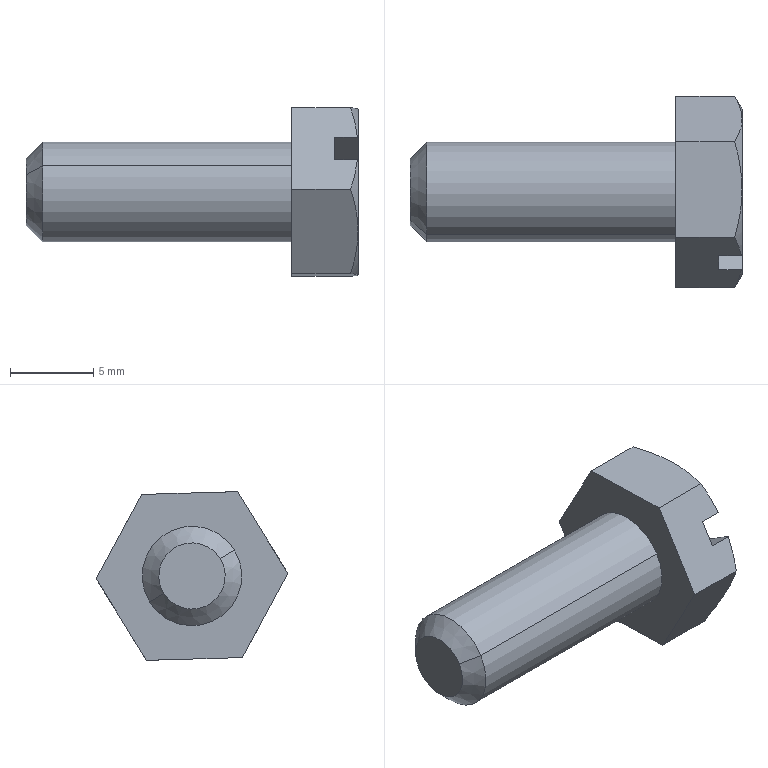Part | SolidWorks | features BaseBody 1 | 1 solid | 23 faces | box 20 x 11.542 x 10.162 mm | volume 766.933 mm3 | plane 13 | cone 8 | cylinder 2 | commonest cylinder face diameters 6 x2
STEP:
#1=CARTESIAN_POINT('',(431.2,61.298,25.05));
#2=VERTEX_POINT('',#1);
#3=CARTESIAN_POINT('',(431.2,64.702,22.95));
#4=VERTEX_POINT('',#3);
#5=CARTESIAN_POINT('',(431.2,63.,24.));
#6=DIRECTION('',(-1.,0.,0.));
#7=DIRECTION('',(0.,-0.8512,0.5248));
#8=AXIS2_PLACEMENT_3D('',#5,#6,#7);
#9=CIRCLE('',#8,2.);
#10=EDGE_CURVE('',#2,#4,#9,.T.);
#11=ORIENTED_EDGE('',*,*,#10,.F.);
#12=CARTESIAN_POINT('',(432.2,60.446,25.574));
#13=VERTEX_POINT('',#12);
#14=CARTESIAN_POINT('',(431.2,61.298,25.05));
#15=DIRECTION('',(0.7071,-0.6019,0.3711));
#16=VECTOR('',#15,1000.);
#17=LINE('',#14,#16);
#18=EDGE_CURVE('',#2,#13,#17,.T.);
#19=ORIENTED_EDGE('',*,*,#18,.T.);
#20=CARTESIAN_POINT('',(432.2,65.554,22.426));
#21=VERTEX_POINT('',#20);
#22=CARTESIAN_POINT('',(432.2,63.,24.));
#23=DIRECTION('',(1.,0.,0.));
#24=DIRECTION('',(0.,-0.8512,0.5248));
#25=AXIS2_PLACEMENT_3D('',#22,#23,#24);
#26=CIRCLE('',#25,3.);
#27=EDGE_CURVE('',#21,#13,#26,.T.);
#28=ORIENTED_EDGE('',*,*,#27,.F.);
#29=CARTESIAN_POINT('',(431.2,64.702,22.95));
#30=DIRECTION('',(0.7071,0.6019,-0.3711));
#31=VECTOR('',#30,1000.);
#32=LINE('',#29,#31);
#33=EDGE_CURVE('',#4,#21,#32,.T.);
#34=ORIENTED_EDGE('',*,*,#33,.F.);
#35=EDGE_LOOP('',(#11,#19,#28,#34));
#36=FACE_OUTER_BOUND('',#35,.T.);
#37=CARTESIAN_POINT('',(431.2,63.,24.));
#38=DIRECTION('',(1.,0.,0.));
#39=DIRECTION('',(0.,0.8512,-0.5248));
#40=AXIS2_PLACEMENT_3D('',#37,#38,#39);
#41=CONICAL_SURFACE('',#40,2.,0.7854);
#42=ADVANCED_FACE('',(#36),#41,.T.);
#43=ORIENTED_EDGE('',*,*,#27,.T.);
#44=CARTESIAN_POINT('',(447.2,60.446,25.574));
#45=VERTEX_POINT('',#44);
#46=CARTESIAN_POINT('',(431.2,60.446,25.574));
#47=DIRECTION('',(1.,0.,0.));
#48=VECTOR('',#47,1000.);
#49=LINE('',#46,#48);
#50=EDGE_CURVE('',#13,#45,#49,.T.);
#51=ORIENTED_EDGE('',*,*,#50,.T.);
#52=CARTESIAN_POINT('',(447.2,65.554,22.426));
#53=VERTEX_POINT('',#52);
#54=CARTESIAN_POINT('',(447.2,63.,24.));
#55=DIRECTION('',(-1.,0.,0.));
#56=DIRECTION('',(0.,-0.8512,0.5248));
#57=AXIS2_PLACEMENT_3D('',#54,#55,#56);
#58=CIRCLE('',#57,3.);
#59=EDGE_CURVE('',#45,#53,#58,.T.);
#60=ORIENTED_EDGE('',*,*,#59,.T.);
#61=CARTESIAN_POINT('',(431.2,65.554,22.426));
#62=DIRECTION('',(1.,0.,0.));
#63=VECTOR('',#62,1000.);
#64=LINE('',#61,#63);
#65=EDGE_CURVE('',#21,#53,#64,.T.);
#66=ORIENTED_EDGE('',*,*,#65,.F.);
#67=EDGE_LOOP('',(#43,#51,#60,#66));
#68=FACE_OUTER_BOUND('',#67,.T.);
#69=CARTESIAN_POINT('',(431.2,63.,24.));
#70=DIRECTION('',(1.,0.,0.));
#71=DIRECTION('',(0.,0.8512,-0.5248));
#72=AXIS2_PLACEMENT_3D('',#69,#70,#71);
#73=CYLINDRICAL_SURFACE('',#72,3.);
#74=ADVANCED_FACE('',(#68),#73,.T.);
#75=CARTESIAN_POINT('',(447.2,66.03,28.915));
#76=VERTEX_POINT('',#75);
#77=CARTESIAN_POINT('',(447.2,68.771,23.833));
#78=VERTEX_POINT('',#77);
#79=CARTESIAN_POINT('',(447.2,68.771,23.833));
#80=DIRECTION('',(0.,0.4748,-0.8801));
#81=VECTOR('',#80,1000.);
#82=LINE('',#79,#81);
#83=EDGE_CURVE('',#76,#78,#82,.T.);
#84=ORIENTED_EDGE('',*,*,#83,.T.);
#85=CARTESIAN_POINT('',(447.2,65.741,18.919));
#86=VERTEX_POINT('',#85);
#87=CARTESIAN_POINT('',(447.2,65.741,18.919));
#88=DIRECTION('',(0.,-0.5248,-0.8512));
#89=VECTOR('',#88,1000.);
#90=LINE('',#87,#89);
#91=EDGE_CURVE('',#78,#86,#90,.T.);
#92=ORIENTED_EDGE('',*,*,#91,.T.);
#93=CARTESIAN_POINT('',(447.2,59.97,19.085));
#94=VERTEX_POINT('',#93);
#95=CARTESIAN_POINT('',(447.2,65.741,18.919));
#96=DIRECTION('',(0.,-0.9996,0.02887));
#97=VECTOR('',#96,1000.);
#98=LINE('',#95,#97);
#99=EDGE_CURVE('',#86,#94,#98,.T.);
#100=ORIENTED_EDGE('',*,*,#99,.T.);
#101=CARTESIAN_POINT('',(447.2,57.229,24.167));
#102=VERTEX_POINT('',#101);
#103=CARTESIAN_POINT('',(447.2,57.229,24.167));
#104=DIRECTION('',(0.,-0.4748,0.8801));
#105=VECTOR('',#104,1000.);
#106=LINE('',#103,#105);
#107=EDGE_CURVE('',#94,#102,#106,.T.);
#108=ORIENTED_EDGE('',*,*,#107,.T.);
#109=CARTESIAN_POINT('',(447.2,60.259,29.081));
#110=VERTEX_POINT('',#109);
#111=CARTESIAN_POINT('',(447.2,57.229,24.167));
#112=DIRECTION('',(0.,0.5248,0.8512));
#113=VECTOR('',#112,1000.);
#114=LINE('',#111,#113);
#115=EDGE_CURVE('',#102,#110,#114,.T.);
#116=ORIENTED_EDGE('',*,*,#115,.T.);
#117=CARTESIAN_POINT('',(447.2,60.259,29.081));
#118=DIRECTION('',(0.,0.9996,-0.02887));
#119=VECTOR('',#118,1000.);
#120=LINE('',#117,#119);
#121=EDGE_CURVE('',#110,#76,#120,.T.);
#122=ORIENTED_EDGE('',*,*,#121,.T.);
#123=EDGE_LOOP('',(#84,#92,#100,#108,#116,#122));
#124=FACE_OUTER_BOUND('',#123,.T.);
#125=CARTESIAN_POINT('',(447.2,63.,24.));
#126=DIRECTION('',(-1.,0.,0.));
#127=DIRECTION('',(0.,-0.8512,0.5248));
#128=AXIS2_PLACEMENT_3D('',#125,#126,#127);
#129=CIRCLE('',#128,3.);
#130=EDGE_CURVE('',#53,#45,#129,.T.);
#131=ORIENTED_EDGE('',*,*,#130,.F.);
#132=ORIENTED_EDGE('',*,*,#59,.F.);
#133=EDGE_LOOP('',(#131,#132));
#134=FACE_BOUND('',#133,.T.);
#135=CARTESIAN_POINT('',(447.2,68.771,23.833));
#136=DIRECTION('',(-1.,0.,0.));
#137=DIRECTION('',(0.,-0.8512,0.5248));
#138=AXIS2_PLACEMENT_3D('',#135,#136,#137);
#139=PLANE('',#138);
#140=ADVANCED_FACE('',(#124,#134),#139,.T.);
#141=CARTESIAN_POINT('',(451.2,62.856,19.002));
#142=VERTEX_POINT('',#141);
#143=CARTESIAN_POINT('',(451.2,66.781,20.729));
#144=VERTEX_POINT('',#143);
#145=CARTESIAN_POINT('',(451.2,63.,24.));
#146=DIRECTION('',(1.,0.,0.));
#147=DIRECTION('',(0.,0.8512,-0.5248));
#148=AXIS2_PLACEMENT_3D('',#145,#146,#147);
#149=CIRCLE('',#148,5.);
#150=EDGE_CURVE('',#142,#144,#149,.T.);
#151=ORIENTED_EDGE('',*,*,#150,.T.);
#152=CARTESIAN_POINT('',(451.2,58.379,25.909));
#153=VERTEX_POINT('',#152);
#154=CARTESIAN_POINT('',(451.2,58.324,25.943));
#155=DIRECTION('',(0.,0.8512,-0.5248));
#156=VECTOR('',#155,1000.);
#157=LINE('',#154,#156);
#158=EDGE_CURVE('',#153,#144,#157,.T.);
#159=ORIENTED_EDGE('',*,*,#158,.F.);
#160=CARTESIAN_POINT('',(451.2,58.6,21.626));
#161=VERTEX_POINT('',#160);
#162=CARTESIAN_POINT('',(451.2,63.,24.));
#163=DIRECTION('',(1.,0.,0.));
#164=DIRECTION('',(0.,0.8512,-0.5248));
#165=AXIS2_PLACEMENT_3D('',#162,#163,#164);
#166=CIRCLE('',#165,5.);
#167=EDGE_CURVE('',#153,#161,#166,.T.);
#168=ORIENTED_EDGE('',*,*,#167,.T.);
#169=CARTESIAN_POINT('',(451.2,63.,24.));
#170=DIRECTION('',(1.,0.,0.));
#171=DIRECTION('',(0.,0.8512,-0.5248));
#172=AXIS2_PLACEMENT_3D('',#169,#170,#171);
#173=CIRCLE('',#172,5.);
#174=EDGE_CURVE('',#161,#142,#173,.T.);
#175=ORIENTED_EDGE('',*,*,#174,.T.);
#176=EDGE_LOOP('',(#151,#159,#168,#175));
#177=FACE_OUTER_BOUND('',#176,.T.);
#178=CARTESIAN_POINT('',(451.2,68.771,23.833));
#179=DIRECTION('',(-1.,0.,0.));
#180=DIRECTION('',(0.,-0.8512,0.5248));
#181=AXIS2_PLACEMENT_3D('',#178,#179,#180);
#182=PLANE('',#181);
#183=ADVANCED_FACE('',(#177),#182,.F.);
#184=CARTESIAN_POINT('',(450.753,68.771,23.833));
#185=VERTEX_POINT('',#184);
#186=CARTESIAN_POINT('',(451.2,67.4,26.374));
#187=VERTEX_POINT('',#186);
#188=CARTESIAN_POINT('',(450.753,68.771,23.833));
#189=CARTESIAN_POINT('',(451.026,68.323,24.665));
#190=CARTESIAN_POINT('',(451.2,67.868,25.508));
#191=CARTESIAN_POINT('',(451.2,67.4,26.374));
#192=B_SPLINE_CURVE_WITH_KNOTS('',3,(#188,#189,#190,#191),.UNSPECIFIED.,.F.,.F.,(4,4),(0.000000238,0.002921),.UNSPECIFIED.);
#193=EDGE_CURVE('',#185,#187,#192,.T.);
#194=ORIENTED_EDGE('',*,*,#193,.F.);
#195=CARTESIAN_POINT('',(447.2,68.771,23.833));
#196=DIRECTION('',(1.,0.,0.));
#197=VECTOR('',#196,1000.);
#198=LINE('',#195,#197);
#199=EDGE_CURVE('',#78,#185,#198,.T.);
#200=ORIENTED_EDGE('',*,*,#199,.F.);
#201=ORIENTED_EDGE('',*,*,#83,.F.);
#202=CARTESIAN_POINT('',(450.753,66.03,28.915));
#203=VERTEX_POINT('',#202);
#204=CARTESIAN_POINT('',(447.2,66.03,28.915));
#205=DIRECTION('',(1.,0.,0.));
#206=VECTOR('',#205,1000.);
#207=LINE('',#204,#206);
#208=EDGE_CURVE('',#76,#203,#207,.T.);
#209=ORIENTED_EDGE('',*,*,#208,.T.);
#210=CARTESIAN_POINT('',(451.2,67.4,26.374));
#211=CARTESIAN_POINT('',(451.2,67.284,26.59));
#212=CARTESIAN_POINT('',(451.189,67.167,26.806));
#213=CARTESIAN_POINT('',(451.149,66.936,27.235));
#214=CARTESIAN_POINT('',(451.118,66.821,27.447));
#215=CARTESIAN_POINT('',(451.002,66.479,28.082));
#216=CARTESIAN_POINT('',(450.889,66.254,28.5));
#217=CARTESIAN_POINT('',(450.753,66.03,28.915));
#218=B_SPLINE_CURVE_WITH_KNOTS('',3,(#210,#211,#212,#213,#214,#215,#216,#217),.UNSPECIFIED.,.F.,.F.,(4,2,2,4),(0.002921,0.003649,0.004376,0.005831),.UNSPECIFIED.);
#219=EDGE_CURVE('',#187,#203,#218,.T.);
#220=ORIENTED_EDGE('',*,*,#219,.F.);
#221=EDGE_LOOP('',(#194,#200,#201,#209,#220));
#222=FACE_OUTER_BOUND('',#221,.T.);
#223=CARTESIAN_POINT('',(447.2,68.771,23.833));
#224=DIRECTION('',(0.,-0.8801,-0.4748));
#225=DIRECTION('',(0.,-0.4748,0.8801));
#226=AXIS2_PLACEMENT_3D('',#223,#224,#225);
#227=PLANE('',#226);
#228=ADVANCED_FACE('',(#222),#227,.F.);
#229=CARTESIAN_POINT('',(450.753,65.741,18.919));
#230=VERTEX_POINT('',#229);
#231=CARTESIAN_POINT('',(451.163,66.836,20.695));
#232=VERTEX_POINT('',#231);
#233=CARTESIAN_POINT('',(450.753,65.741,18.919));
#234=CARTESIAN_POINT('',(450.852,65.92,19.209));
#235=CARTESIAN_POINT('',(450.939,66.103,19.505));
#236=CARTESIAN_POINT('',(451.079,66.468,20.098));
#237=CARTESIAN_POINT('',(451.131,66.652,20.396));
#238=CARTESIAN_POINT('',(451.163,66.836,20.695));
#239=B_SPLINE_CURVE_WITH_KNOTS('',3,(#233,#234,#235,#236,#237,#238),.UNSPECIFIED.,.F.,.F.,(4,2,4),(0.005386,0.006447,0.007508),.UNSPECIFIED.);
#240=EDGE_CURVE('',#230,#232,#239,.T.);
#241=ORIENTED_EDGE('',*,*,#240,.F.);
#242=CARTESIAN_POINT('',(447.2,65.741,18.919));
#243=DIRECTION('',(1.,0.,0.));
#244=VECTOR('',#243,1000.);
#245=LINE('',#242,#244);
#246=EDGE_CURVE('',#86,#230,#245,.T.);
#247=ORIENTED_EDGE('',*,*,#246,.F.);
#248=ORIENTED_EDGE('',*,*,#91,.F.);
#249=ORIENTED_EDGE('',*,*,#199,.T.);
#250=CARTESIAN_POINT('',(451.163,67.676,22.057));
#251=VERTEX_POINT('',#250);
#252=CARTESIAN_POINT('',(451.163,67.676,22.057));
#253=CARTESIAN_POINT('',(451.098,68.051,22.665));
#254=CARTESIAN_POINT('',(450.95,68.414,23.254));
#255=CARTESIAN_POINT('',(450.753,68.771,23.833));
#256=B_SPLINE_CURVE_WITH_KNOTS('',3,(#252,#253,#254,#255),.UNSPECIFIED.,.F.,.F.,(4,4),(0.009104,0.01123),.UNSPECIFIED.);
#257=EDGE_CURVE('',#251,#185,#256,.T.);
#258=ORIENTED_EDGE('',*,*,#257,.F.);
#259=CARTESIAN_POINT('',(449.8,67.676,22.057));
#260=VERTEX_POINT('',#259);
#261=CARTESIAN_POINT('',(449.8,67.676,22.057));
#262=DIRECTION('',(1.,0.,0.));
#263=VECTOR('',#262,1000.);
#264=LINE('',#261,#263);
#265=EDGE_CURVE('',#260,#251,#264,.T.);
#266=ORIENTED_EDGE('',*,*,#265,.F.);
#267=CARTESIAN_POINT('',(449.8,66.836,20.695));
#268=VERTEX_POINT('',#267);
#269=CARTESIAN_POINT('',(449.8,67.676,22.057));
#270=DIRECTION('',(0.,0.5248,0.8512));
#271=VECTOR('',#270,1000.);
#272=LINE('',#269,#271);
#273=EDGE_CURVE('',#268,#260,#272,.T.);
#274=ORIENTED_EDGE('',*,*,#273,.F.);
#275=CARTESIAN_POINT('',(449.8,66.836,20.695));
#276=DIRECTION('',(1.,0.,0.));
#277=VECTOR('',#276,1000.);
#278=LINE('',#275,#277);
#279=EDGE_CURVE('',#268,#232,#278,.T.);
#280=ORIENTED_EDGE('',*,*,#279,.T.);
#281=EDGE_LOOP('',(#241,#247,#248,#249,#258,#266,#274,#280));
#282=FACE_OUTER_BOUND('',#281,.T.);
#283=CARTESIAN_POINT('',(447.2,65.741,18.919));
#284=DIRECTION('',(0.,-0.8512,0.5248));
#285=DIRECTION('',(0.,0.5248,0.8512));
#286=AXIS2_PLACEMENT_3D('',#283,#284,#285);
#287=PLANE('',#286);
#288=ADVANCED_FACE('',(#282),#287,.F.);
#289=CARTESIAN_POINT('',(450.753,59.97,19.085));
#290=VERTEX_POINT('',#289);
#291=CARTESIAN_POINT('',(450.753,59.97,19.085));
#292=CARTESIAN_POINT('',(451.026,60.914,19.058));
#293=CARTESIAN_POINT('',(451.2,61.872,19.03));
#294=CARTESIAN_POINT('',(451.2,62.856,19.002));
#295=B_SPLINE_CURVE_WITH_KNOTS('',3,(#291,#292,#293,#294),.UNSPECIFIED.,.F.,.F.,(4,4),(0.000000238,0.002921),.UNSPECIFIED.);
#296=EDGE_CURVE('',#290,#142,#295,.T.);
#297=ORIENTED_EDGE('',*,*,#296,.F.);
#298=CARTESIAN_POINT('',(447.2,59.97,19.085));
#299=DIRECTION('',(1.,0.,0.));
#300=VECTOR('',#299,1000.);
#301=LINE('',#298,#300);
#302=EDGE_CURVE('',#94,#290,#301,.T.);
#303=ORIENTED_EDGE('',*,*,#302,.F.);
#304=ORIENTED_EDGE('',*,*,#99,.F.);
#305=ORIENTED_EDGE('',*,*,#246,.T.);
#306=CARTESIAN_POINT('',(451.2,62.856,19.002));
#307=CARTESIAN_POINT('',(451.2,63.101,18.995));
#308=CARTESIAN_POINT('',(451.189,63.347,18.988));
#309=CARTESIAN_POINT('',(451.149,63.833,18.974));
#310=CARTESIAN_POINT('',(451.118,64.075,18.967));
#311=CARTESIAN_POINT('',(451.002,64.796,18.946));
#312=CARTESIAN_POINT('',(450.889,65.27,18.932));
#313=CARTESIAN_POINT('',(450.753,65.741,18.919));
#314=B_SPLINE_CURVE_WITH_KNOTS('',3,(#306,#307,#308,#309,#310,#311,#312,#313),.UNSPECIFIED.,.F.,.F.,(4,2,2,4),(0.002921,0.003649,0.004376,0.005831),.UNSPECIFIED.);
#315=EDGE_CURVE('',#142,#230,#314,.T.);
#316=ORIENTED_EDGE('',*,*,#315,.F.);
#317=EDGE_LOOP('',(#297,#303,#304,#305,#316));
#318=FACE_OUTER_BOUND('',#317,.T.);
#319=CARTESIAN_POINT('',(447.2,65.741,18.919));
#320=DIRECTION('',(0.,0.02887,0.9996));
#321=DIRECTION('',(0.,0.9996,-0.02887));
#322=AXIS2_PLACEMENT_3D('',#319,#320,#321);
#323=PLANE('',#322);
#324=ADVANCED_FACE('',(#318),#323,.F.);
#325=CARTESIAN_POINT('',(450.753,57.229,24.167));
#326=VERTEX_POINT('',#325);
#327=CARTESIAN_POINT('',(450.753,57.229,24.167));
#328=CARTESIAN_POINT('',(451.026,57.677,23.335));
#329=CARTESIAN_POINT('',(451.2,58.132,22.492));
#330=CARTESIAN_POINT('',(451.2,58.6,21.626));
#331=B_SPLINE_CURVE_WITH_KNOTS('',3,(#327,#328,#329,#330),.UNSPECIFIED.,.F.,.F.,(4,4),(0.000000238,0.002921),.UNSPECIFIED.);
#332=EDGE_CURVE('',#326,#161,#331,.T.);
#333=ORIENTED_EDGE('',*,*,#332,.F.);
#334=CARTESIAN_POINT('',(447.2,57.229,24.167));
#335=DIRECTION('',(1.,0.,0.));
#336=VECTOR('',#335,1000.);
#337=LINE('',#334,#336);
#338=EDGE_CURVE('',#102,#326,#337,.T.);
#339=ORIENTED_EDGE('',*,*,#338,.F.);
#340=ORIENTED_EDGE('',*,*,#107,.F.);
#341=ORIENTED_EDGE('',*,*,#302,.T.);
#342=CARTESIAN_POINT('',(451.2,58.6,21.626));
#343=CARTESIAN_POINT('',(451.2,58.716,21.41));
#344=CARTESIAN_POINT('',(451.189,58.833,21.194));
#345=CARTESIAN_POINT('',(451.149,59.064,20.765));
#346=CARTESIAN_POINT('',(451.118,59.179,20.553));
#347=CARTESIAN_POINT('',(451.002,59.521,19.918));
#348=CARTESIAN_POINT('',(450.889,59.746,19.5));
#349=CARTESIAN_POINT('',(450.753,59.97,19.085));
#350=B_SPLINE_CURVE_WITH_KNOTS('',3,(#342,#343,#344,#345,#346,#347,#348,#349),.UNSPECIFIED.,.F.,.F.,(4,2,2,4),(0.002921,0.003649,0.004376,0.005831),.UNSPECIFIED.);
#351=EDGE_CURVE('',#161,#290,#350,.T.);
#352=ORIENTED_EDGE('',*,*,#351,.F.);
#353=EDGE_LOOP('',(#333,#339,#340,#341,#352));
#354=FACE_OUTER_BOUND('',#353,.T.);
#355=CARTESIAN_POINT('',(447.2,57.229,24.167));
#356=DIRECTION('',(0.,0.8801,0.4748));
#357=DIRECTION('',(0.,0.4748,-0.8801));
#358=AXIS2_PLACEMENT_3D('',#355,#356,#357);
#359=PLANE('',#358);
#360=ADVANCED_FACE('',(#354),#359,.F.);
#361=CARTESIAN_POINT('',(450.753,60.259,29.081));
#362=VERTEX_POINT('',#361);
#363=CARTESIAN_POINT('',(451.163,59.164,27.305));
#364=VERTEX_POINT('',#363);
#365=CARTESIAN_POINT('',(450.753,60.259,29.081));
#366=CARTESIAN_POINT('',(450.95,59.902,28.502));
#367=CARTESIAN_POINT('',(451.098,59.538,27.913));
#368=CARTESIAN_POINT('',(451.163,59.164,27.305));
#369=B_SPLINE_CURVE_WITH_KNOTS('',3,(#365,#366,#367,#368),.UNSPECIFIED.,.F.,.F.,(4,4),(0.0154,0.01752),.UNSPECIFIED.);
#370=EDGE_CURVE('',#362,#364,#369,.T.);
#371=ORIENTED_EDGE('',*,*,#370,.F.);
#372=CARTESIAN_POINT('',(447.2,60.259,29.081));
#373=DIRECTION('',(1.,0.,0.));
#374=VECTOR('',#373,1000.);
#375=LINE('',#372,#374);
#376=EDGE_CURVE('',#110,#362,#375,.T.);
#377=ORIENTED_EDGE('',*,*,#376,.F.);
#378=ORIENTED_EDGE('',*,*,#115,.F.);
#379=ORIENTED_EDGE('',*,*,#338,.T.);
#380=CARTESIAN_POINT('',(451.163,58.324,25.943));
#381=VERTEX_POINT('',#380);
#382=CARTESIAN_POINT('',(451.163,58.324,25.943));
#383=CARTESIAN_POINT('',(451.131,58.139,25.644));
#384=CARTESIAN_POINT('',(451.079,57.956,25.346));
#385=CARTESIAN_POINT('',(450.939,57.59,24.753));
#386=CARTESIAN_POINT('',(450.852,57.408,24.457));
#387=CARTESIAN_POINT('',(450.753,57.229,24.167));
#388=B_SPLINE_CURVE_WITH_KNOTS('',3,(#382,#383,#384,#385,#386,#387),.UNSPECIFIED.,.F.,.F.,(4,2,4),(0.01912,0.02018,0.02124),.UNSPECIFIED.);
#389=EDGE_CURVE('',#381,#326,#388,.T.);
#390=ORIENTED_EDGE('',*,*,#389,.F.);
#391=CARTESIAN_POINT('',(449.8,58.324,25.943));
#392=VERTEX_POINT('',#391);
#393=CARTESIAN_POINT('',(449.8,58.324,25.943));
#394=DIRECTION('',(1.,0.,0.));
#395=VECTOR('',#394,1000.);
#396=LINE('',#393,#395);
#397=EDGE_CURVE('',#392,#381,#396,.T.);
#398=ORIENTED_EDGE('',*,*,#397,.F.);
#399=CARTESIAN_POINT('',(449.8,59.164,27.305));
#400=VERTEX_POINT('',#399);
#401=CARTESIAN_POINT('',(449.8,58.324,25.943));
#402=DIRECTION('',(0.,-0.5248,-0.8512));
#403=VECTOR('',#402,1000.);
#404=LINE('',#401,#403);
#405=EDGE_CURVE('',#400,#392,#404,.T.);
#406=ORIENTED_EDGE('',*,*,#405,.F.);
#407=CARTESIAN_POINT('',(449.8,59.164,27.305));
#408=DIRECTION('',(1.,0.,0.));
#409=VECTOR('',#408,1000.);
#410=LINE('',#407,#409);
#411=EDGE_CURVE('',#400,#364,#410,.T.);
#412=ORIENTED_EDGE('',*,*,#411,.T.);
#413=EDGE_LOOP('',(#371,#377,#378,#379,#390,#398,#406,#412));
#414=FACE_OUTER_BOUND('',#413,.T.);
#415=CARTESIAN_POINT('',(447.2,57.229,24.167));
#416=DIRECTION('',(0.,0.8512,-0.5248));
#417=DIRECTION('',(-1.,0.,0.));
#418=AXIS2_PLACEMENT_3D('',#415,#416,#417);
#419=PLANE('',#418);
#420=ADVANCED_FACE('',(#414),#419,.F.);
#421=CARTESIAN_POINT('',(451.2,63.144,28.998));
#422=VERTEX_POINT('',#421);
#423=CARTESIAN_POINT('',(450.753,66.03,28.915));
#424=CARTESIAN_POINT('',(451.026,65.086,28.942));
#425=CARTESIAN_POINT('',(451.2,64.128,28.97));
#426=CARTESIAN_POINT('',(451.2,63.144,28.998));
#427=B_SPLINE_CURVE_WITH_KNOTS('',3,(#423,#424,#425,#426),.UNSPECIFIED.,.F.,.F.,(4,4),(0.000000238,0.002921),.UNSPECIFIED.);
#428=EDGE_CURVE('',#203,#422,#427,.T.);
#429=ORIENTED_EDGE('',*,*,#428,.F.);
#430=ORIENTED_EDGE('',*,*,#208,.F.);
#431=ORIENTED_EDGE('',*,*,#121,.F.);
#432=ORIENTED_EDGE('',*,*,#376,.T.);
#433=CARTESIAN_POINT('',(451.2,63.144,28.998));
#434=CARTESIAN_POINT('',(451.2,62.899,29.005));
#435=CARTESIAN_POINT('',(451.189,62.653,29.012));
#436=CARTESIAN_POINT('',(451.149,62.167,29.026));
#437=CARTESIAN_POINT('',(451.118,61.925,29.033));
#438=CARTESIAN_POINT('',(451.002,61.204,29.054));
#439=CARTESIAN_POINT('',(450.889,60.73,29.068));
#440=CARTESIAN_POINT('',(450.753,60.259,29.081));
#441=B_SPLINE_CURVE_WITH_KNOTS('',3,(#433,#434,#435,#436,#437,#438,#439,#440),.UNSPECIFIED.,.F.,.F.,(4,2,2,4),(0.002921,0.003649,0.004376,0.005831),.UNSPECIFIED.);
#442=EDGE_CURVE('',#422,#362,#441,.T.);
#443=ORIENTED_EDGE('',*,*,#442,.F.);
#444=EDGE_LOOP('',(#429,#430,#431,#432,#443));
#445=FACE_OUTER_BOUND('',#444,.T.);
#446=CARTESIAN_POINT('',(447.2,60.259,29.081));
#447=DIRECTION('',(0.,-0.02887,-0.9996));
#448=DIRECTION('',(0.,-0.9996,0.02887));
#449=AXIS2_PLACEMENT_3D('',#446,#447,#448);
#450=PLANE('',#449);
#451=ADVANCED_FACE('',(#445),#450,.F.);
#452=CARTESIAN_POINT('',(451.2,59.219,27.271));
#453=VERTEX_POINT('',#452);
#454=CARTESIAN_POINT('',(451.2,63.,24.));
#455=DIRECTION('',(1.,0.,0.));
#456=DIRECTION('',(0.,0.8512,-0.5248));
#457=AXIS2_PLACEMENT_3D('',#454,#455,#456);
#458=CIRCLE('',#457,5.);
#459=EDGE_CURVE('',#422,#453,#458,.T.);
#460=ORIENTED_EDGE('',*,*,#459,.T.);
#461=CARTESIAN_POINT('',(451.2,67.621,22.091));
#462=VERTEX_POINT('',#461);
#463=CARTESIAN_POINT('',(451.2,59.164,27.305));
#464=DIRECTION('',(0.,-0.8512,0.5248));
#465=VECTOR('',#464,1000.);
#466=LINE('',#463,#465);
#467=EDGE_CURVE('',#462,#453,#466,.T.);
#468=ORIENTED_EDGE('',*,*,#467,.F.);
#469=CARTESIAN_POINT('',(451.2,63.,24.));
#470=DIRECTION('',(1.,0.,0.));
#471=DIRECTION('',(0.,0.8512,-0.5248));
#472=AXIS2_PLACEMENT_3D('',#469,#470,#471);
#473=CIRCLE('',#472,5.);
#474=EDGE_CURVE('',#462,#187,#473,.T.);
#475=ORIENTED_EDGE('',*,*,#474,.T.);
#476=CARTESIAN_POINT('',(451.2,63.,24.));
#477=DIRECTION('',(1.,0.,0.));
#478=DIRECTION('',(0.,0.8512,-0.5248));
#479=AXIS2_PLACEMENT_3D('',#476,#477,#478);
#480=CIRCLE('',#479,5.);
#481=EDGE_CURVE('',#187,#422,#480,.T.);
#482=ORIENTED_EDGE('',*,*,#481,.T.);
#483=EDGE_LOOP('',(#460,#468,#475,#482));
#484=FACE_OUTER_BOUND('',#483,.T.);
#485=CARTESIAN_POINT('',(451.2,68.771,23.833));
#486=DIRECTION('',(-1.,0.,0.));
#487=DIRECTION('',(0.,-0.8512,0.5248));
#488=AXIS2_PLACEMENT_3D('',#485,#486,#487);
#489=PLANE('',#488);
#490=ADVANCED_FACE('',(#484),#489,.F.);
#491=CARTESIAN_POINT('',(451.163,66.836,20.695));
#492=CARTESIAN_POINT('',(451.176,66.818,20.706));
#493=CARTESIAN_POINT('',(451.188,66.8,20.718));
#494=CARTESIAN_POINT('',(451.2,66.781,20.729));
#495=B_SPLINE_CURVE_WITH_KNOTS('',3,(#491,#492,#493,#494),.UNSPECIFIED.,.F.,.F.,(4,4),(0.006986,0.00706),.UNSPECIFIED.);
#496=EDGE_CURVE('',#232,#144,#495,.T.);
#497=ORIENTED_EDGE('',*,*,#496,.F.);
#498=ORIENTED_EDGE('',*,*,#279,.F.);
#499=CARTESIAN_POINT('',(449.8,58.324,25.943));
#500=DIRECTION('',(0.,0.8512,-0.5248));
#501=VECTOR('',#500,1000.);
#502=LINE('',#499,#501);
#503=EDGE_CURVE('',#392,#268,#502,.T.);
#504=ORIENTED_EDGE('',*,*,#503,.F.);
#505=ORIENTED_EDGE('',*,*,#397,.T.);
#506=CARTESIAN_POINT('',(451.2,58.379,25.909));
#507=CARTESIAN_POINT('',(451.188,58.361,25.92));
#508=CARTESIAN_POINT('',(451.176,58.342,25.932));
#509=CARTESIAN_POINT('',(451.163,58.324,25.943));
#510=B_SPLINE_CURVE_WITH_KNOTS('',3,(#506,#507,#508,#509),.UNSPECIFIED.,.F.,.F.,(4,4),(0.01814,0.01822),.UNSPECIFIED.);
#511=EDGE_CURVE('',#153,#381,#510,.T.);
#512=ORIENTED_EDGE('',*,*,#511,.F.);
#513=ORIENTED_EDGE('',*,*,#158,.T.);
#514=EDGE_LOOP('',(#497,#498,#504,#505,#512,#513));
#515=FACE_OUTER_BOUND('',#514,.T.);
#516=CARTESIAN_POINT('',(449.8,58.324,25.943));
#517=DIRECTION('',(0.,-0.5248,-0.8512));
#518=DIRECTION('',(1.,0.,0.));
#519=AXIS2_PLACEMENT_3D('',#516,#517,#518);
#520=PLANE('',#519);
#521=ADVANCED_FACE('',(#515),#520,.F.);
#522=CARTESIAN_POINT('',(451.163,59.164,27.305));
#523=CARTESIAN_POINT('',(451.176,59.182,27.294));
#524=CARTESIAN_POINT('',(451.188,59.2,27.282));
#525=CARTESIAN_POINT('',(451.2,59.219,27.271));
#526=B_SPLINE_CURVE_WITH_KNOTS('',3,(#522,#523,#524,#525),.UNSPECIFIED.,.F.,.F.,(4,4),(0.006986,0.00706),.UNSPECIFIED.);
#527=EDGE_CURVE('',#364,#453,#526,.T.);
#528=ORIENTED_EDGE('',*,*,#527,.F.);
#529=ORIENTED_EDGE('',*,*,#411,.F.);
#530=CARTESIAN_POINT('',(449.8,59.164,27.305));
#531=DIRECTION('',(0.,-0.8512,0.5248));
#532=VECTOR('',#531,1000.);
#533=LINE('',#530,#532);
#534=EDGE_CURVE('',#260,#400,#533,.T.);
#535=ORIENTED_EDGE('',*,*,#534,.F.);
#536=ORIENTED_EDGE('',*,*,#265,.T.);
#537=CARTESIAN_POINT('',(451.2,67.621,22.091));
#538=CARTESIAN_POINT('',(451.188,67.639,22.08));
#539=CARTESIAN_POINT('',(451.176,67.658,22.068));
#540=CARTESIAN_POINT('',(451.163,67.676,22.057));
#541=B_SPLINE_CURVE_WITH_KNOTS('',3,(#537,#538,#539,#540),.UNSPECIFIED.,.F.,.F.,(4,4),(0.01814,0.01822),.UNSPECIFIED.);
#542=EDGE_CURVE('',#462,#251,#541,.T.);
#543=ORIENTED_EDGE('',*,*,#542,.F.);
#544=ORIENTED_EDGE('',*,*,#467,.T.);
#545=EDGE_LOOP('',(#528,#529,#535,#536,#543,#544));
#546=FACE_OUTER_BOUND('',#545,.T.);
#547=CARTESIAN_POINT('',(449.8,59.164,27.305));
#548=DIRECTION('',(0.,0.5248,0.8512));
#549=DIRECTION('',(-1.,0.,0.));
#550=AXIS2_PLACEMENT_3D('',#547,#548,#549);
#551=PLANE('',#550);
#552=ADVANCED_FACE('',(#546),#551,.F.);
#553=ORIENTED_EDGE('',*,*,#273,.T.);
#554=ORIENTED_EDGE('',*,*,#534,.T.);
#555=ORIENTED_EDGE('',*,*,#405,.T.);
#556=ORIENTED_EDGE('',*,*,#503,.T.);
#557=EDGE_LOOP('',(#553,#554,#555,#556));
#558=FACE_OUTER_BOUND('',#557,.T.);
#559=CARTESIAN_POINT('',(449.8,66.836,20.695));
#560=DIRECTION('',(1.,0.,0.));
#561=DIRECTION('',(0.,0.8512,-0.5248));
#562=AXIS2_PLACEMENT_3D('',#559,#560,#561);
#563=PLANE('',#562);
#564=ADVANCED_FACE('',(#558),#563,.T.);
#565=ORIENTED_EDGE('',*,*,#193,.T.);
#566=ORIENTED_EDGE('',*,*,#474,.F.);
#567=ORIENTED_EDGE('',*,*,#542,.T.);
#568=ORIENTED_EDGE('',*,*,#257,.T.);
#569=EDGE_LOOP('',(#565,#566,#567,#568));
#570=FACE_OUTER_BOUND('',#569,.T.);
#571=CARTESIAN_POINT('',(451.2,63.,24.));
#572=DIRECTION('',(-1.,0.,0.));
#573=DIRECTION('',(0.,0.8512,-0.5248));
#574=AXIS2_PLACEMENT_3D('',#571,#572,#573);
#575=CONICAL_SURFACE('',#574,5.,1.047);
#576=ADVANCED_FACE('',(#570),#575,.T.);
#577=ORIENTED_EDGE('',*,*,#527,.T.);
#578=ORIENTED_EDGE('',*,*,#459,.F.);
#579=ORIENTED_EDGE('',*,*,#442,.T.);
#580=ORIENTED_EDGE('',*,*,#370,.T.);
#581=EDGE_LOOP('',(#577,#578,#579,#580));
#582=FACE_OUTER_BOUND('',#581,.T.);
#583=CARTESIAN_POINT('',(451.2,63.,24.));
#584=DIRECTION('',(-1.,0.,0.));
#585=DIRECTION('',(0.,0.8512,-0.5248));
#586=AXIS2_PLACEMENT_3D('',#583,#584,#585);
#587=CONICAL_SURFACE('',#586,5.,1.047);
#588=ADVANCED_FACE('',(#582),#587,.T.);
#589=ORIENTED_EDGE('',*,*,#332,.T.);
#590=ORIENTED_EDGE('',*,*,#167,.F.);
#591=ORIENTED_EDGE('',*,*,#511,.T.);
#592=ORIENTED_EDGE('',*,*,#389,.T.);
#593=EDGE_LOOP('',(#589,#590,#591,#592));
#594=FACE_OUTER_BOUND('',#593,.T.);
#595=CARTESIAN_POINT('',(451.2,63.,24.));
#596=DIRECTION('',(-1.,0.,0.));
#597=DIRECTION('',(0.,0.8512,-0.5248));
#598=AXIS2_PLACEMENT_3D('',#595,#596,#597);
#599=CONICAL_SURFACE('',#598,5.,1.047);
#600=ADVANCED_FACE('',(#594),#599,.T.);
#601=ORIENTED_EDGE('',*,*,#496,.T.);
#602=ORIENTED_EDGE('',*,*,#150,.F.);
#603=ORIENTED_EDGE('',*,*,#315,.T.);
#604=ORIENTED_EDGE('',*,*,#240,.T.);
#605=EDGE_LOOP('',(#601,#602,#603,#604));
#606=FACE_OUTER_BOUND('',#605,.T.);
#607=CARTESIAN_POINT('',(451.2,63.,24.));
#608=DIRECTION('',(-1.,0.,0.));
#609=DIRECTION('',(0.,0.8512,-0.5248));
#610=AXIS2_PLACEMENT_3D('',#607,#608,#609);
#611=CONICAL_SURFACE('',#610,5.,1.047);
#612=ADVANCED_FACE('',(#606),#611,.T.);
#613=ORIENTED_EDGE('',*,*,#428,.T.);
#614=ORIENTED_EDGE('',*,*,#481,.F.);
#615=ORIENTED_EDGE('',*,*,#219,.T.);
#616=EDGE_LOOP('',(#613,#614,#615));
#617=FACE_OUTER_BOUND('',#616,.T.);
#618=CARTESIAN_POINT('',(451.2,63.,24.));
#619=DIRECTION('',(-1.,0.,0.));
#620=DIRECTION('',(0.,0.8512,-0.5248));
#621=AXIS2_PLACEMENT_3D('',#618,#619,#620);
#622=CONICAL_SURFACE('',#621,5.,1.047);
#623=ADVANCED_FACE('',(#617),#622,.T.);
#624=ORIENTED_EDGE('',*,*,#296,.T.);
#625=ORIENTED_EDGE('',*,*,#174,.F.);
#626=ORIENTED_EDGE('',*,*,#351,.T.);
#627=EDGE_LOOP('',(#624,#625,#626));
#628=FACE_OUTER_BOUND('',#627,.T.);
#629=CARTESIAN_POINT('',(451.2,63.,24.));
#630=DIRECTION('',(-1.,0.,0.));
#631=DIRECTION('',(0.,0.8512,-0.5248));
#632=AXIS2_PLACEMENT_3D('',#629,#630,#631);
#633=CONICAL_SURFACE('',#632,5.,1.047);
#634=ADVANCED_FACE('',(#628),#633,.T.);
#635=ORIENTED_EDGE('',*,*,#50,.F.);
#636=CARTESIAN_POINT('',(432.2,63.,24.));
#637=DIRECTION('',(1.,0.,0.));
#638=DIRECTION('',(0.,-0.8512,0.5248));
#639=AXIS2_PLACEMENT_3D('',#636,#637,#638);
#640=CIRCLE('',#639,3.);
#641=EDGE_CURVE('',#13,#21,#640,.T.);
#642=ORIENTED_EDGE('',*,*,#641,.T.);
#643=ORIENTED_EDGE('',*,*,#65,.T.);
#644=ORIENTED_EDGE('',*,*,#130,.T.);
#645=EDGE_LOOP('',(#635,#642,#643,#644));
#646=FACE_OUTER_BOUND('',#645,.T.);
#647=CARTESIAN_POINT('',(431.2,63.,24.));
#648=DIRECTION('',(1.,0.,0.));
#649=DIRECTION('',(0.,0.8512,-0.5248));
#650=AXIS2_PLACEMENT_3D('',#647,#648,#649);
#651=CYLINDRICAL_SURFACE('',#650,3.);
#652=ADVANCED_FACE('',(#646),#651,.T.);
#653=CARTESIAN_POINT('',(431.2,63.,24.));
#654=DIRECTION('',(-1.,0.,0.));
#655=DIRECTION('',(0.,-0.8512,0.5248));
#656=AXIS2_PLACEMENT_3D('',#653,#654,#655);
#657=CIRCLE('',#656,2.);
#658=EDGE_CURVE('',#4,#2,#657,.T.);
#659=ORIENTED_EDGE('',*,*,#658,.T.);
#660=ORIENTED_EDGE('',*,*,#10,.T.);
#661=EDGE_LOOP('',(#659,#660));
#662=FACE_OUTER_BOUND('',#661,.T.);
#663=CARTESIAN_POINT('',(431.2,63.,24.));
#664=DIRECTION('',(-1.,0.,0.));
#665=DIRECTION('',(0.,-0.8512,0.5248));
#666=AXIS2_PLACEMENT_3D('',#663,#664,#665);
#667=PLANE('',#666);
#668=ADVANCED_FACE('',(#662),#667,.T.);
#669=ORIENTED_EDGE('',*,*,#18,.F.);
#670=ORIENTED_EDGE('',*,*,#658,.F.);
#671=ORIENTED_EDGE('',*,*,#33,.T.);
#672=ORIENTED_EDGE('',*,*,#641,.F.);
#673=EDGE_LOOP('',(#669,#670,#671,#672));
#674=FACE_OUTER_BOUND('',#673,.T.);
#675=CARTESIAN_POINT('',(431.2,63.,24.));
#676=DIRECTION('',(1.,0.,0.));
#677=DIRECTION('',(0.,0.8512,-0.5248));
#678=AXIS2_PLACEMENT_3D('',#675,#676,#677);
#679=CONICAL_SURFACE('',#678,2.,0.7854);
#680=ADVANCED_FACE('',(#674),#679,.T.);
#681=CLOSED_SHELL('',(#42,#74,#140,#183,#228,#288,#324,#360,#420,#451,#490,#521,#552,#564,#576,#588,#600,#612,#623,#634,#652,#668,#680));
#682=MANIFOLD_SOLID_BREP('',#681);
#683=CARTESIAN_POINT('',(0.,0.,0.));
#684=DIRECTION('',(0.,0.,1.));
#685=DIRECTION('',(1.,0.,0.));
#686=AXIS2_PLACEMENT_3D('',#683,#684,#685);
#687=(LENGTH_UNIT()NAMED_UNIT(*)SI_UNIT(.MILLI.,.METRE.));
#688=UNCERTAINTY_MEASURE_WITH_UNIT(LENGTH_MEASURE(0.00001),#687,'','');
#689=(NAMED_UNIT(*)PLANE_ANGLE_UNIT()SI_UNIT($,.RADIAN.));
#690=(NAMED_UNIT(*)SI_UNIT($,.STERADIAN.)SOLID_ANGLE_UNIT());
#691=(GEOMETRIC_REPRESENTATION_CONTEXT(3)GLOBAL_UNCERTAINTY_ASSIGNED_CONTEXT((#688))GLOBAL_UNIT_ASSIGNED_CONTEXT((#687,#689,#690))REPRESENTATION_CONTEXT('',''));
#692=ADVANCED_BREP_SHAPE_REPRESENTATION('',(#682,#686),#691);